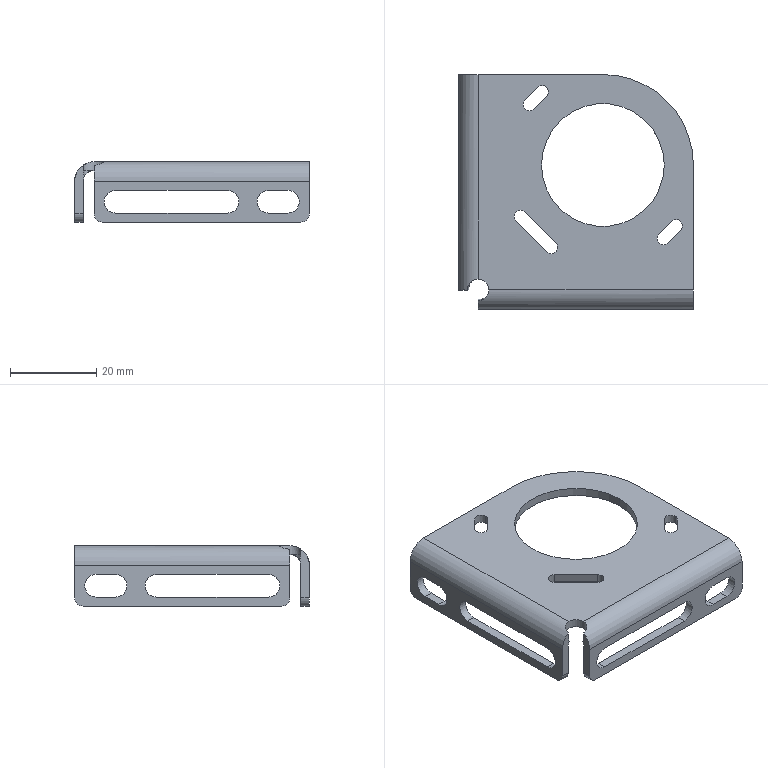Part | STEP file | 00396465_ADAPTER_HMZAS-PG21 | 1 solid | 57 faces | box 54.5 x 54.5 x 14 mm | volume 5523 mm3 | cylinder 29 | plane 26 | spline 2 | commonest cylinder face diameters 3 x9 5.3 x8 4 x4 5 x3 9 x2 28.5 x2